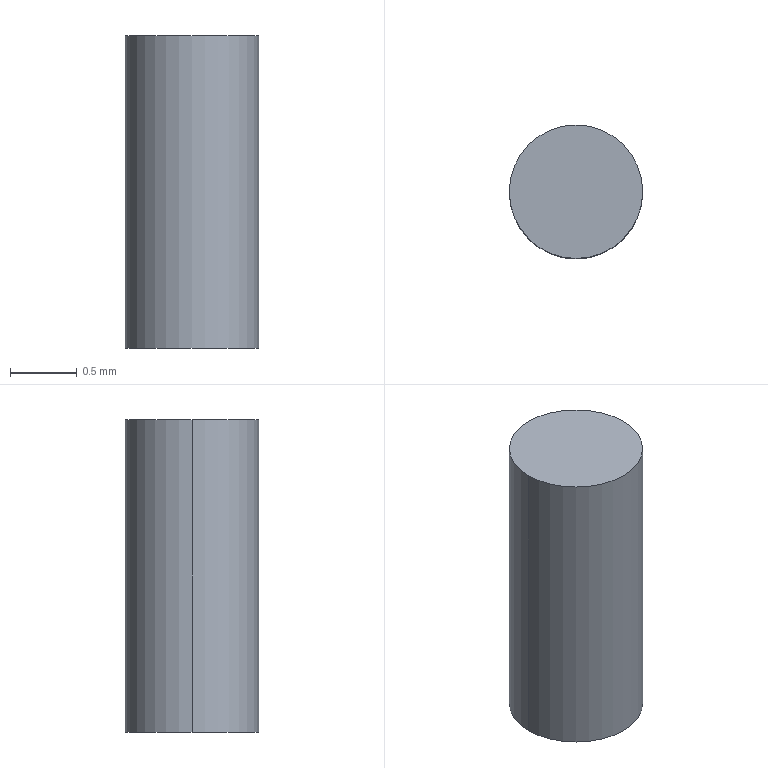Part | SolidWorks | features BaseBody 1 | 1 solid | 4 faces | box 1 x 1 x 2.34 mm | volume 1.838 mm3 | cylinder 2 | plane 2 | commonest cylinder face diameters 1 x2
STEP:
#1=CARTESIAN_POINT('',(566.72,76.38,70.213));
#2=VERTEX_POINT('',#1);
#3=CARTESIAN_POINT('',(565.72,76.38,70.213));
#4=VERTEX_POINT('',#3);
#5=CARTESIAN_POINT('',(566.22,76.38,70.213));
#6=DIRECTION('',(0.,0.,1.));
#7=DIRECTION('',(1.,0.,0.));
#8=AXIS2_PLACEMENT_3D('',#5,#6,#7);
#9=CIRCLE('',#8,0.5);
#10=EDGE_CURVE('',#2,#4,#9,.T.);
#11=ORIENTED_EDGE('',*,*,#10,.T.);
#12=CARTESIAN_POINT('',(565.72,76.38,72.553));
#13=VERTEX_POINT('',#12);
#14=CARTESIAN_POINT('',(565.72,76.38,71.553));
#15=DIRECTION('',(0.,0.,1.));
#16=VECTOR('',#15,1000.);
#17=LINE('',#14,#16);
#18=EDGE_CURVE('',#4,#13,#17,.T.);
#19=ORIENTED_EDGE('',*,*,#18,.T.);
#20=CARTESIAN_POINT('',(566.72,76.38,72.553));
#21=VERTEX_POINT('',#20);
#22=CARTESIAN_POINT('',(566.22,76.38,72.553));
#23=DIRECTION('',(0.,0.,-1.));
#24=DIRECTION('',(1.,0.,0.));
#25=AXIS2_PLACEMENT_3D('',#22,#23,#24);
#26=CIRCLE('',#25,0.5);
#27=EDGE_CURVE('',#13,#21,#26,.T.);
#28=ORIENTED_EDGE('',*,*,#27,.T.);
#29=CARTESIAN_POINT('',(566.72,76.38,71.553));
#30=DIRECTION('',(0.,0.,1.));
#31=VECTOR('',#30,1000.);
#32=LINE('',#29,#31);
#33=EDGE_CURVE('',#2,#21,#32,.T.);
#34=ORIENTED_EDGE('',*,*,#33,.F.);
#35=EDGE_LOOP('',(#11,#19,#28,#34));
#36=FACE_OUTER_BOUND('',#35,.T.);
#37=CARTESIAN_POINT('',(566.22,76.38,71.553));
#38=DIRECTION('',(0.,0.,1.));
#39=DIRECTION('',(1.,0.,0.));
#40=AXIS2_PLACEMENT_3D('',#37,#38,#39);
#41=CYLINDRICAL_SURFACE('',#40,0.5);
#42=ADVANCED_FACE('',(#36),#41,.T.);
#43=ORIENTED_EDGE('',*,*,#18,.F.);
#44=CARTESIAN_POINT('',(566.22,76.38,70.213));
#45=DIRECTION('',(0.,0.,1.));
#46=DIRECTION('',(1.,0.,0.));
#47=AXIS2_PLACEMENT_3D('',#44,#45,#46);
#48=CIRCLE('',#47,0.5);
#49=EDGE_CURVE('',#4,#2,#48,.T.);
#50=ORIENTED_EDGE('',*,*,#49,.T.);
#51=ORIENTED_EDGE('',*,*,#33,.T.);
#52=CARTESIAN_POINT('',(566.22,76.38,72.553));
#53=DIRECTION('',(0.,0.,-1.));
#54=DIRECTION('',(1.,0.,0.));
#55=AXIS2_PLACEMENT_3D('',#52,#53,#54);
#56=CIRCLE('',#55,0.5);
#57=EDGE_CURVE('',#21,#13,#56,.T.);
#58=ORIENTED_EDGE('',*,*,#57,.T.);
#59=EDGE_LOOP('',(#43,#50,#51,#58));
#60=FACE_OUTER_BOUND('',#59,.T.);
#61=CARTESIAN_POINT('',(566.22,76.38,71.553));
#62=DIRECTION('',(0.,0.,1.));
#63=DIRECTION('',(1.,0.,0.));
#64=AXIS2_PLACEMENT_3D('',#61,#62,#63);
#65=CYLINDRICAL_SURFACE('',#64,0.5);
#66=ADVANCED_FACE('',(#60),#65,.T.);
#67=ORIENTED_EDGE('',*,*,#57,.F.);
#68=ORIENTED_EDGE('',*,*,#27,.F.);
#69=EDGE_LOOP('',(#67,#68));
#70=FACE_OUTER_BOUND('',#69,.T.);
#71=CARTESIAN_POINT('',(566.22,76.38,72.553));
#72=DIRECTION('',(0.,0.,1.));
#73=DIRECTION('',(1.,0.,0.));
#74=AXIS2_PLACEMENT_3D('',#71,#72,#73);
#75=PLANE('',#74);
#76=ADVANCED_FACE('',(#70),#75,.T.);
#77=ORIENTED_EDGE('',*,*,#10,.F.);
#78=ORIENTED_EDGE('',*,*,#49,.F.);
#79=EDGE_LOOP('',(#77,#78));
#80=FACE_OUTER_BOUND('',#79,.T.);
#81=CARTESIAN_POINT('',(566.22,76.38,70.213));
#82=DIRECTION('',(0.,0.,-1.));
#83=DIRECTION('',(-1.,0.,0.));
#84=AXIS2_PLACEMENT_3D('',#81,#82,#83);
#85=PLANE('',#84);
#86=ADVANCED_FACE('',(#80),#85,.T.);
#87=CLOSED_SHELL('',(#42,#66,#76,#86));
#88=MANIFOLD_SOLID_BREP('',#87);
#89=CARTESIAN_POINT('',(0.,0.,0.));
#90=DIRECTION('',(0.,0.,1.));
#91=DIRECTION('',(1.,0.,0.));
#92=AXIS2_PLACEMENT_3D('',#89,#90,#91);
#93=(LENGTH_UNIT()NAMED_UNIT(*)SI_UNIT(.MILLI.,.METRE.));
#94=UNCERTAINTY_MEASURE_WITH_UNIT(LENGTH_MEASURE(0.00001),#93,'','');
#95=(NAMED_UNIT(*)PLANE_ANGLE_UNIT()SI_UNIT($,.RADIAN.));
#96=(NAMED_UNIT(*)SI_UNIT($,.STERADIAN.)SOLID_ANGLE_UNIT());
#97=(GEOMETRIC_REPRESENTATION_CONTEXT(3)GLOBAL_UNCERTAINTY_ASSIGNED_CONTEXT((#94))GLOBAL_UNIT_ASSIGNED_CONTEXT((#93,#95,#96))REPRESENTATION_CONTEXT('',''));
#98=ADVANCED_BREP_SHAPE_REPRESENTATION('',(#88,#92),#97);